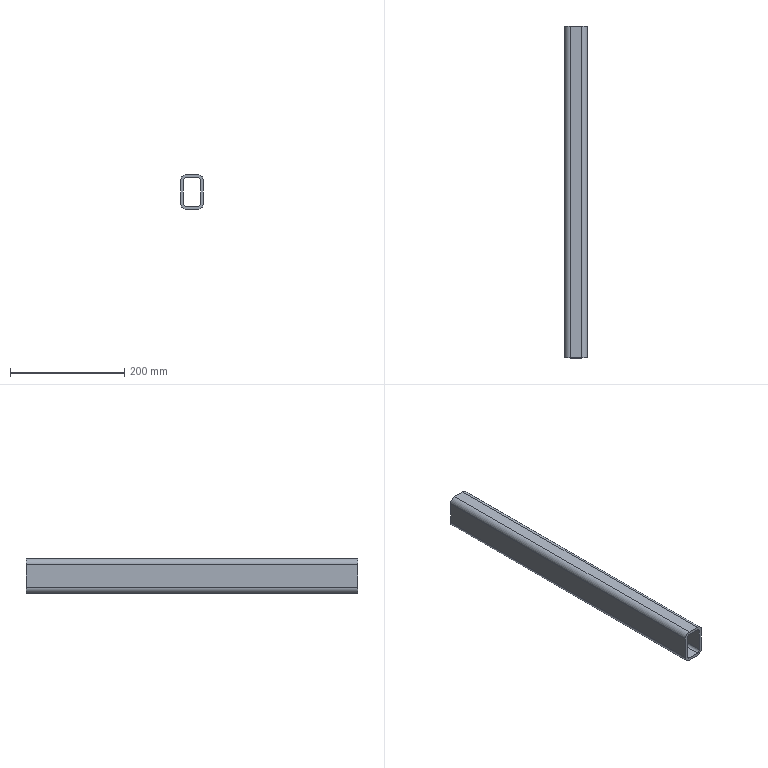Part | STEP file | HL4GD-1.30.109 base frame front crossmember--20251212 | 1 solid | 18 faces | box 40 x 580 x 60 mm | volume 484659 mm3 | plane 10 | cylinder 8 | commonest cylinder face diameters 10 x4 20 x4
STEP:
#1=CARTESIAN_POINT('',(0.,0.,0.));
#2=DIRECTION('',(0.,0.,1.));
#3=DIRECTION('',(1.,0.,0.));
#4=AXIS2_PLACEMENT_3D('',#1,#2,#3);
#5=CARTESIAN_POINT('',(2335.,1110.,410.));
#6=VERTEX_POINT('',#5);
#7=CARTESIAN_POINT('',(2330.,1110.,415.));
#8=VERTEX_POINT('',#7);
#9=CARTESIAN_POINT('',(2335.,1110.,415.));
#10=DIRECTION('',(0.,1.,0.));
#11=DIRECTION('',(-1.,0.,0.));
#12=AXIS2_PLACEMENT_3D('',#9,#10,#11);
#13=CIRCLE('',#12,5.);
#14=CARTESIAN_POINT('',(2335.,530.,415.));
#15=DIRECTION('',(0.,1.,0.));
#16=DIRECTION('',(-1.,0.,0.));
#17=AXIS2_PLACEMENT_3D('',#14,#15,#16);
#18=CYLINDRICAL_SURFACE('',#17,5.);
#19=CARTESIAN_POINT('',(0.,580.));
#20=DIRECTION('',(1.,0.));
#21=VECTOR('',#20,1.);
#22=LINE('',#19,#21);
#23=(GEOMETRIC_REPRESENTATION_CONTEXT(2)PARAMETRIC_REPRESENTATION_CONTEXT()REPRESENTATION_CONTEXT('',''));
#24=DEFINITIONAL_REPRESENTATION('',(#22),#23);
#25=PCURVE('',#18,#24);
#26=CARTESIAN_POINT('',(2148.93,1110.,281.07));
#27=DIRECTION('',(0.,1.,0.));
#28=DIRECTION('',(-1.,0.,0.));
#29=AXIS2_PLACEMENT_3D('',#26,#27,#28);
#30=PLANE('',#29);
#31=CARTESIAN_POINT('',(-186.07,133.93));
#32=DIRECTION('',(1.,0.));
#33=AXIS2_PLACEMENT_2D('',#31,#32);
#34=CIRCLE('',#33,5.);
#35=(GEOMETRIC_REPRESENTATION_CONTEXT(2)PARAMETRIC_REPRESENTATION_CONTEXT()REPRESENTATION_CONTEXT('',''));
#36=DEFINITIONAL_REPRESENTATION('',(#34),#35);
#37=PCURVE('',#30,#36);
#38=SURFACE_CURVE('',#13,(#25,#37),.PCURVE_S1.);
#39=EDGE_CURVE('',#6,#8,#38,.T.);
#40=ORIENTED_EDGE('',*,*,#39,.F.);
#41=CARTESIAN_POINT('',(2335.,530.,410.));
#42=VERTEX_POINT('',#41);
#43=CARTESIAN_POINT('',(2335.,530.,410.));
#44=DIRECTION('',(0.,1.,0.));
#45=VECTOR('',#44,1.);
#46=LINE('',#43,#45);
#47=CARTESIAN_POINT('',(4.712,0.));
#48=DIRECTION('',(0.,1.));
#49=VECTOR('',#48,1.);
#50=LINE('',#47,#49);
#51=(GEOMETRIC_REPRESENTATION_CONTEXT(2)PARAMETRIC_REPRESENTATION_CONTEXT()REPRESENTATION_CONTEXT('',''));
#52=DEFINITIONAL_REPRESENTATION('',(#50),#51);
#53=PCURVE('',#18,#52);
#54=CARTESIAN_POINT('',(2355.,530.,410.));
#55=DIRECTION('',(0.,0.,1.));
#56=DIRECTION('',(1.,0.,0.));
#57=AXIS2_PLACEMENT_3D('',#54,#55,#56);
#58=PLANE('',#57);
#59=CARTESIAN_POINT('',(-20.,0.));
#60=DIRECTION('',(0.,1.));
#61=VECTOR('',#60,1.);
#62=LINE('',#59,#61);
#63=(GEOMETRIC_REPRESENTATION_CONTEXT(2)PARAMETRIC_REPRESENTATION_CONTEXT()REPRESENTATION_CONTEXT('',''));
#64=DEFINITIONAL_REPRESENTATION('',(#62),#63);
#65=PCURVE('',#58,#64);
#66=SURFACE_CURVE('',#46,(#53,#65),.PCURVE_S1.);
#67=EDGE_CURVE('',#42,#6,#66,.T.);
#68=ORIENTED_EDGE('',*,*,#67,.F.);
#69=CARTESIAN_POINT('',(2330.,530.,415.));
#70=VERTEX_POINT('',#69);
#71=CARTESIAN_POINT('',(2335.,530.,415.));
#72=DIRECTION('',(0.,1.,0.));
#73=DIRECTION('',(-1.,0.,0.));
#74=AXIS2_PLACEMENT_3D('',#71,#72,#73);
#75=CIRCLE('',#74,5.);
#76=CARTESIAN_POINT('',(0.,0.));
#77=DIRECTION('',(1.,0.));
#78=VECTOR('',#77,1.);
#79=LINE('',#76,#78);
#80=(GEOMETRIC_REPRESENTATION_CONTEXT(2)PARAMETRIC_REPRESENTATION_CONTEXT()REPRESENTATION_CONTEXT('',''));
#81=DEFINITIONAL_REPRESENTATION('',(#79),#80);
#82=PCURVE('',#18,#81);
#83=CARTESIAN_POINT('',(2148.93,530.,281.07));
#84=DIRECTION('',(0.,1.,0.));
#85=DIRECTION('',(-1.,0.,0.));
#86=AXIS2_PLACEMENT_3D('',#83,#84,#85);
#87=PLANE('',#86);
#88=CARTESIAN_POINT('',(-186.07,133.93));
#89=DIRECTION('',(1.,0.));
#90=AXIS2_PLACEMENT_2D('',#88,#89);
#91=CIRCLE('',#90,5.);
#92=(GEOMETRIC_REPRESENTATION_CONTEXT(2)PARAMETRIC_REPRESENTATION_CONTEXT()REPRESENTATION_CONTEXT('',''));
#93=DEFINITIONAL_REPRESENTATION('',(#91),#92);
#94=PCURVE('',#87,#93);
#95=SURFACE_CURVE('',#75,(#82,#94),.PCURVE_S1.);
#96=EDGE_CURVE('',#42,#70,#95,.T.);
#97=ORIENTED_EDGE('',*,*,#96,.T.);
#98=CARTESIAN_POINT('',(2330.,530.,415.));
#99=DIRECTION('',(0.,1.,0.));
#100=VECTOR('',#99,1.);
#101=LINE('',#98,#100);
#102=CARTESIAN_POINT('',(6.283,0.));
#103=DIRECTION('',(0.,1.));
#104=VECTOR('',#103,1.);
#105=LINE('',#102,#104);
#106=(GEOMETRIC_REPRESENTATION_CONTEXT(2)PARAMETRIC_REPRESENTATION_CONTEXT()REPRESENTATION_CONTEXT('',''));
#107=DEFINITIONAL_REPRESENTATION('',(#105),#106);
#108=PCURVE('',#18,#107);
#109=CARTESIAN_POINT('',(2330.,530.,415.));
#110=DIRECTION('',(1.,0.,0.));
#111=DIRECTION('',(0.,0.,-1.));
#112=AXIS2_PLACEMENT_3D('',#109,#110,#111);
#113=PLANE('',#112);
#114=CARTESIAN_POINT('',(0.,0.));
#115=DIRECTION('',(0.,1.));
#116=VECTOR('',#115,1.);
#117=LINE('',#114,#116);
#118=(GEOMETRIC_REPRESENTATION_CONTEXT(2)PARAMETRIC_REPRESENTATION_CONTEXT()REPRESENTATION_CONTEXT('',''));
#119=DEFINITIONAL_REPRESENTATION('',(#117),#118);
#120=PCURVE('',#113,#119);
#121=SURFACE_CURVE('',#101,(#108,#120),.PCURVE_S1.);
#122=EDGE_CURVE('',#70,#8,#121,.T.);
#123=ORIENTED_EDGE('',*,*,#122,.T.);
#124=EDGE_LOOP('',(#40,#68,#97,#123));
#125=FACE_BOUND('',#124,.F.);
#126=ADVANCED_FACE('',(#125),#18,.F.);
#127=ORIENTED_EDGE('',*,*,#67,.F.);
#128=CARTESIAN_POINT('',(2355.,530.,410.));
#129=VERTEX_POINT('',#128);
#130=CARTESIAN_POINT('',(2355.,530.,410.));
#131=DIRECTION('',(1.,0.,0.));
#132=VECTOR('',#131,1.);
#133=LINE('',#130,#132);
#134=CARTESIAN_POINT('',(0.,0.));
#135=DIRECTION('',(1.,0.));
#136=VECTOR('',#135,1.);
#137=LINE('',#134,#136);
#138=(GEOMETRIC_REPRESENTATION_CONTEXT(2)PARAMETRIC_REPRESENTATION_CONTEXT()REPRESENTATION_CONTEXT('',''));
#139=DEFINITIONAL_REPRESENTATION('',(#137),#138);
#140=PCURVE('',#58,#139);
#141=CARTESIAN_POINT('',(-206.07,128.93));
#142=DIRECTION('',(-1.,0.));
#143=VECTOR('',#142,1.);
#144=LINE('',#141,#143);
#145=(GEOMETRIC_REPRESENTATION_CONTEXT(2)PARAMETRIC_REPRESENTATION_CONTEXT()REPRESENTATION_CONTEXT('',''));
#146=DEFINITIONAL_REPRESENTATION('',(#144),#145);
#147=PCURVE('',#87,#146);
#148=SURFACE_CURVE('',#133,(#140,#147),.PCURVE_S1.);
#149=EDGE_CURVE('',#42,#129,#148,.T.);
#150=ORIENTED_EDGE('',*,*,#149,.T.);
#151=CARTESIAN_POINT('',(2355.,1110.,410.));
#152=VERTEX_POINT('',#151);
#153=CARTESIAN_POINT('',(2355.,530.,410.));
#154=DIRECTION('',(0.,1.,0.));
#155=VECTOR('',#154,1.);
#156=LINE('',#153,#155);
#157=CARTESIAN_POINT('',(0.,0.));
#158=DIRECTION('',(0.,1.));
#159=VECTOR('',#158,1.);
#160=LINE('',#157,#159);
#161=(GEOMETRIC_REPRESENTATION_CONTEXT(2)PARAMETRIC_REPRESENTATION_CONTEXT()REPRESENTATION_CONTEXT('',''));
#162=DEFINITIONAL_REPRESENTATION('',(#160),#161);
#163=PCURVE('',#58,#162);
#164=CARTESIAN_POINT('',(2355.,530.,415.));
#165=DIRECTION('',(0.,1.,0.));
#166=DIRECTION('',(-1.,0.,0.));
#167=AXIS2_PLACEMENT_3D('',#164,#165,#166);
#168=CYLINDRICAL_SURFACE('',#167,5.);
#169=CARTESIAN_POINT('',(4.712,0.));
#170=DIRECTION('',(0.,1.));
#171=VECTOR('',#170,1.);
#172=LINE('',#169,#171);
#173=(GEOMETRIC_REPRESENTATION_CONTEXT(2)PARAMETRIC_REPRESENTATION_CONTEXT()REPRESENTATION_CONTEXT('',''));
#174=DEFINITIONAL_REPRESENTATION('',(#172),#173);
#175=PCURVE('',#168,#174);
#176=SURFACE_CURVE('',#156,(#163,#175),.PCURVE_S1.);
#177=EDGE_CURVE('',#129,#152,#176,.T.);
#178=ORIENTED_EDGE('',*,*,#177,.T.);
#179=CARTESIAN_POINT('',(2148.93,1110.,410.));
#180=DIRECTION('',(1.,0.,0.));
#181=VECTOR('',#180,1.);
#182=LINE('',#179,#181);
#183=CARTESIAN_POINT('',(-206.07,580.));
#184=DIRECTION('',(1.,0.));
#185=VECTOR('',#184,1.);
#186=LINE('',#183,#185);
#187=(GEOMETRIC_REPRESENTATION_CONTEXT(2)PARAMETRIC_REPRESENTATION_CONTEXT()REPRESENTATION_CONTEXT('',''));
#188=DEFINITIONAL_REPRESENTATION('',(#186),#187);
#189=PCURVE('',#58,#188);
#190=CARTESIAN_POINT('',(0.,128.93));
#191=DIRECTION('',(-1.,0.));
#192=VECTOR('',#191,1.);
#193=LINE('',#190,#192);
#194=(GEOMETRIC_REPRESENTATION_CONTEXT(2)PARAMETRIC_REPRESENTATION_CONTEXT()REPRESENTATION_CONTEXT('',''));
#195=DEFINITIONAL_REPRESENTATION('',(#193),#194);
#196=PCURVE('',#30,#195);
#197=SURFACE_CURVE('',#182,(#189,#196),.PCURVE_S1.);
#198=EDGE_CURVE('',#6,#152,#197,.T.);
#199=ORIENTED_EDGE('',*,*,#198,.F.);
#200=EDGE_LOOP('',(#127,#150,#178,#199));
#201=FACE_BOUND('',#200,.T.);
#202=ADVANCED_FACE('',(#201),#58,.T.);
#203=CARTESIAN_POINT('',(2360.,1110.,415.));
#204=VERTEX_POINT('',#203);
#205=CARTESIAN_POINT('',(2355.,1110.,415.));
#206=DIRECTION('',(0.,-1.,0.));
#207=DIRECTION('',(-1.,0.,0.));
#208=AXIS2_PLACEMENT_3D('',#205,#206,#207);
#209=CIRCLE('',#208,5.);
#210=CARTESIAN_POINT('',(6.283,580.));
#211=DIRECTION('',(-1.,0.));
#212=VECTOR('',#211,1.);
#213=LINE('',#210,#212);
#214=(GEOMETRIC_REPRESENTATION_CONTEXT(2)PARAMETRIC_REPRESENTATION_CONTEXT()REPRESENTATION_CONTEXT('',''));
#215=DEFINITIONAL_REPRESENTATION('',(#213),#214);
#216=PCURVE('',#168,#215);
#217=CARTESIAN_POINT('',(-201.07,133.93));
#218=CARTESIAN_POINT('',(-201.07,125.27));
#219=CARTESIAN_POINT('',(-208.57,129.6));
#220=CARTESIAN_POINT('',(-216.07,133.93));
#221=CARTESIAN_POINT('',(-208.57,138.261));
#222=CARTESIAN_POINT('',(-201.07,142.591));
#223=CARTESIAN_POINT('',(-201.07,133.93));
#224=(BOUNDED_CURVE()B_SPLINE_CURVE(2,(#217,#218,#219,#220,#221,#222,#223),.UNSPECIFIED.,.T.,.F.)B_SPLINE_CURVE_WITH_KNOTS((1,2,2,2,2,1),(-2.094,0.,2.094,4.189,6.283,8.378),.UNSPECIFIED.)CURVE()GEOMETRIC_REPRESENTATION_ITEM()RATIONAL_B_SPLINE_CURVE((1.,0.5,1.,0.5,1.,0.5,1.))REPRESENTATION_ITEM(''));
#225=(GEOMETRIC_REPRESENTATION_CONTEXT(2)PARAMETRIC_REPRESENTATION_CONTEXT()REPRESENTATION_CONTEXT('',''));
#226=DEFINITIONAL_REPRESENTATION('',(#224),#225);
#227=PCURVE('',#30,#226);
#228=SURFACE_CURVE('',#209,(#216,#227),.PCURVE_S1.);
#229=EDGE_CURVE('',#152,#204,#228,.T.);
#230=ORIENTED_EDGE('',*,*,#229,.T.);
#231=CARTESIAN_POINT('',(2360.,530.,415.));
#232=VERTEX_POINT('',#231);
#233=CARTESIAN_POINT('',(2360.,530.,415.));
#234=DIRECTION('',(0.,1.,0.));
#235=VECTOR('',#234,1.);
#236=LINE('',#233,#235);
#237=CARTESIAN_POINT('',(3.142,0.));
#238=DIRECTION('',(0.,1.));
#239=VECTOR('',#238,1.);
#240=LINE('',#237,#239);
#241=(GEOMETRIC_REPRESENTATION_CONTEXT(2)PARAMETRIC_REPRESENTATION_CONTEXT()REPRESENTATION_CONTEXT('',''));
#242=DEFINITIONAL_REPRESENTATION('',(#240),#241);
#243=PCURVE('',#168,#242);
#244=CARTESIAN_POINT('',(2360.,530.,455.));
#245=DIRECTION('',(-1.,0.,0.));
#246=DIRECTION('',(0.,0.,1.));
#247=AXIS2_PLACEMENT_3D('',#244,#245,#246);
#248=PLANE('',#247);
#249=CARTESIAN_POINT('',(-40.,0.));
#250=DIRECTION('',(0.,1.));
#251=VECTOR('',#250,1.);
#252=LINE('',#249,#251);
#253=(GEOMETRIC_REPRESENTATION_CONTEXT(2)PARAMETRIC_REPRESENTATION_CONTEXT()REPRESENTATION_CONTEXT('',''));
#254=DEFINITIONAL_REPRESENTATION('',(#252),#253);
#255=PCURVE('',#248,#254);
#256=SURFACE_CURVE('',#236,(#243,#255),.PCURVE_S1.);
#257=EDGE_CURVE('',#232,#204,#256,.T.);
#258=ORIENTED_EDGE('',*,*,#257,.F.);
#259=CARTESIAN_POINT('',(2355.,530.,415.));
#260=DIRECTION('',(0.,-1.,0.));
#261=DIRECTION('',(-1.,0.,0.));
#262=AXIS2_PLACEMENT_3D('',#259,#260,#261);
#263=CIRCLE('',#262,5.);
#264=CARTESIAN_POINT('',(6.283,0.));
#265=DIRECTION('',(-1.,0.));
#266=VECTOR('',#265,1.);
#267=LINE('',#264,#266);
#268=(GEOMETRIC_REPRESENTATION_CONTEXT(2)PARAMETRIC_REPRESENTATION_CONTEXT()REPRESENTATION_CONTEXT('',''));
#269=DEFINITIONAL_REPRESENTATION('',(#267),#268);
#270=PCURVE('',#168,#269);
#271=CARTESIAN_POINT('',(-201.07,133.93));
#272=CARTESIAN_POINT('',(-201.07,125.27));
#273=CARTESIAN_POINT('',(-208.57,129.6));
#274=CARTESIAN_POINT('',(-216.07,133.93));
#275=CARTESIAN_POINT('',(-208.57,138.261));
#276=CARTESIAN_POINT('',(-201.07,142.591));
#277=CARTESIAN_POINT('',(-201.07,133.93));
#278=(BOUNDED_CURVE()B_SPLINE_CURVE(2,(#271,#272,#273,#274,#275,#276,#277),.UNSPECIFIED.,.T.,.F.)B_SPLINE_CURVE_WITH_KNOTS((1,2,2,2,2,1),(-2.094,0.,2.094,4.189,6.283,8.378),.UNSPECIFIED.)CURVE()GEOMETRIC_REPRESENTATION_ITEM()RATIONAL_B_SPLINE_CURVE((1.,0.5,1.,0.5,1.,0.5,1.))REPRESENTATION_ITEM(''));
#279=(GEOMETRIC_REPRESENTATION_CONTEXT(2)PARAMETRIC_REPRESENTATION_CONTEXT()REPRESENTATION_CONTEXT('',''));
#280=DEFINITIONAL_REPRESENTATION('',(#278),#279);
#281=PCURVE('',#87,#280);
#282=SURFACE_CURVE('',#263,(#270,#281),.PCURVE_S1.);
#283=EDGE_CURVE('',#129,#232,#282,.T.);
#284=ORIENTED_EDGE('',*,*,#283,.F.);
#285=ORIENTED_EDGE('',*,*,#177,.T.);
#286=EDGE_LOOP('',(#230,#258,#284,#285));
#287=FACE_BOUND('',#286,.F.);
#288=ADVANCED_FACE('',(#287),#168,.F.);
#289=ORIENTED_EDGE('',*,*,#257,.F.);
#290=CARTESIAN_POINT('',(2360.,530.,455.));
#291=VERTEX_POINT('',#290);
#292=CARTESIAN_POINT('',(2360.,530.,455.));
#293=DIRECTION('',(0.,0.,-1.));
#294=VECTOR('',#293,1.);
#295=LINE('',#292,#294);
#296=CARTESIAN_POINT('',(0.,0.));
#297=DIRECTION('',(-1.,0.));
#298=VECTOR('',#297,1.);
#299=LINE('',#296,#298);
#300=(GEOMETRIC_REPRESENTATION_CONTEXT(2)PARAMETRIC_REPRESENTATION_CONTEXT()REPRESENTATION_CONTEXT('',''));
#301=DEFINITIONAL_REPRESENTATION('',(#299),#300);
#302=PCURVE('',#248,#301);
#303=CARTESIAN_POINT('',(-211.07,173.93));
#304=DIRECTION('',(0.,-1.));
#305=VECTOR('',#304,1.);
#306=LINE('',#303,#305);
#307=(GEOMETRIC_REPRESENTATION_CONTEXT(2)PARAMETRIC_REPRESENTATION_CONTEXT()REPRESENTATION_CONTEXT('',''));
#308=DEFINITIONAL_REPRESENTATION('',(#306),#307);
#309=PCURVE('',#87,#308);
#310=SURFACE_CURVE('',#295,(#302,#309),.PCURVE_S1.);
#311=EDGE_CURVE('',#291,#232,#310,.T.);
#312=ORIENTED_EDGE('',*,*,#311,.F.);
#313=CARTESIAN_POINT('',(2360.,1110.,455.));
#314=VERTEX_POINT('',#313);
#315=CARTESIAN_POINT('',(2360.,530.,455.));
#316=DIRECTION('',(0.,1.,0.));
#317=VECTOR('',#316,1.);
#318=LINE('',#315,#317);
#319=CARTESIAN_POINT('',(0.,0.));
#320=DIRECTION('',(0.,1.));
#321=VECTOR('',#320,1.);
#322=LINE('',#319,#321);
#323=(GEOMETRIC_REPRESENTATION_CONTEXT(2)PARAMETRIC_REPRESENTATION_CONTEXT()REPRESENTATION_CONTEXT('',''));
#324=DEFINITIONAL_REPRESENTATION('',(#322),#323);
#325=PCURVE('',#248,#324);
#326=CARTESIAN_POINT('',(2355.,530.,455.));
#327=DIRECTION('',(0.,1.,0.));
#328=DIRECTION('',(-1.,0.,0.));
#329=AXIS2_PLACEMENT_3D('',#326,#327,#328);
#330=CYLINDRICAL_SURFACE('',#329,5.);
#331=CARTESIAN_POINT('',(3.142,0.));
#332=DIRECTION('',(0.,1.));
#333=VECTOR('',#332,1.);
#334=LINE('',#331,#333);
#335=(GEOMETRIC_REPRESENTATION_CONTEXT(2)PARAMETRIC_REPRESENTATION_CONTEXT()REPRESENTATION_CONTEXT('',''));
#336=DEFINITIONAL_REPRESENTATION('',(#334),#335);
#337=PCURVE('',#330,#336);
#338=SURFACE_CURVE('',#318,(#325,#337),.PCURVE_S1.);
#339=EDGE_CURVE('',#291,#314,#338,.T.);
#340=ORIENTED_EDGE('',*,*,#339,.T.);
#341=CARTESIAN_POINT('',(2360.,1110.,281.07));
#342=DIRECTION('',(0.,0.,-1.));
#343=VECTOR('',#342,1.);
#344=LINE('',#341,#343);
#345=CARTESIAN_POINT('',(-173.93,580.));
#346=DIRECTION('',(-1.,0.));
#347=VECTOR('',#346,1.);
#348=LINE('',#345,#347);
#349=(GEOMETRIC_REPRESENTATION_CONTEXT(2)PARAMETRIC_REPRESENTATION_CONTEXT()REPRESENTATION_CONTEXT('',''));
#350=DEFINITIONAL_REPRESENTATION('',(#348),#349);
#351=PCURVE('',#248,#350);
#352=CARTESIAN_POINT('',(-211.07,0.));
#353=DIRECTION('',(0.,-1.));
#354=VECTOR('',#353,1.);
#355=LINE('',#352,#354);
#356=(GEOMETRIC_REPRESENTATION_CONTEXT(2)PARAMETRIC_REPRESENTATION_CONTEXT()REPRESENTATION_CONTEXT('',''));
#357=DEFINITIONAL_REPRESENTATION('',(#355),#356);
#358=PCURVE('',#30,#357);
#359=SURFACE_CURVE('',#344,(#351,#358),.PCURVE_S1.);
#360=EDGE_CURVE('',#314,#204,#359,.T.);
#361=ORIENTED_EDGE('',*,*,#360,.T.);
#362=EDGE_LOOP('',(#289,#312,#340,#361));
#363=FACE_BOUND('',#362,.T.);
#364=ADVANCED_FACE('',(#363),#248,.T.);
#365=CARTESIAN_POINT('',(2355.,1110.,460.));
#366=VERTEX_POINT('',#365);
#367=CARTESIAN_POINT('',(2355.,1110.,455.));
#368=DIRECTION('',(0.,1.,0.));
#369=DIRECTION('',(-1.,0.,0.));
#370=AXIS2_PLACEMENT_3D('',#367,#368,#369);
#371=CIRCLE('',#370,5.);
#372=CARTESIAN_POINT('',(0.,580.));
#373=DIRECTION('',(1.,0.));
#374=VECTOR('',#373,1.);
#375=LINE('',#372,#374);
#376=(GEOMETRIC_REPRESENTATION_CONTEXT(2)PARAMETRIC_REPRESENTATION_CONTEXT()REPRESENTATION_CONTEXT('',''));
#377=DEFINITIONAL_REPRESENTATION('',(#375),#376);
#378=PCURVE('',#330,#377);
#379=CARTESIAN_POINT('',(-206.07,173.93));
#380=DIRECTION('',(1.,0.));
#381=AXIS2_PLACEMENT_2D('',#379,#380);
#382=CIRCLE('',#381,5.);
#383=(GEOMETRIC_REPRESENTATION_CONTEXT(2)PARAMETRIC_REPRESENTATION_CONTEXT()REPRESENTATION_CONTEXT('',''));
#384=DEFINITIONAL_REPRESENTATION('',(#382),#383);
#385=PCURVE('',#30,#384);
#386=SURFACE_CURVE('',#371,(#378,#385),.PCURVE_S1.);
#387=EDGE_CURVE('',#366,#314,#386,.T.);
#388=ORIENTED_EDGE('',*,*,#387,.F.);
#389=CARTESIAN_POINT('',(2355.,530.,460.));
#390=VERTEX_POINT('',#389);
#391=CARTESIAN_POINT('',(2355.,530.,460.));
#392=DIRECTION('',(0.,1.,0.));
#393=VECTOR('',#392,1.);
#394=LINE('',#391,#393);
#395=CARTESIAN_POINT('',(1.571,0.));
#396=DIRECTION('',(0.,1.));
#397=VECTOR('',#396,1.);
#398=LINE('',#395,#397);
#399=(GEOMETRIC_REPRESENTATION_CONTEXT(2)PARAMETRIC_REPRESENTATION_CONTEXT()REPRESENTATION_CONTEXT('',''));
#400=DEFINITIONAL_REPRESENTATION('',(#398),#399);
#401=PCURVE('',#330,#400);
#402=CARTESIAN_POINT('',(2335.,530.,460.));
#403=DIRECTION('',(0.,0.,-1.));
#404=DIRECTION('',(-1.,0.,0.));
#405=AXIS2_PLACEMENT_3D('',#402,#403,#404);
#406=PLANE('',#405);
#407=CARTESIAN_POINT('',(-20.,0.));
#408=DIRECTION('',(0.,1.));
#409=VECTOR('',#408,1.);
#410=LINE('',#407,#409);
#411=(GEOMETRIC_REPRESENTATION_CONTEXT(2)PARAMETRIC_REPRESENTATION_CONTEXT()REPRESENTATION_CONTEXT('',''));
#412=DEFINITIONAL_REPRESENTATION('',(#410),#411);
#413=PCURVE('',#406,#412);
#414=SURFACE_CURVE('',#394,(#401,#413),.PCURVE_S1.);
#415=EDGE_CURVE('',#390,#366,#414,.T.);
#416=ORIENTED_EDGE('',*,*,#415,.F.);
#417=CARTESIAN_POINT('',(2355.,530.,455.));
#418=DIRECTION('',(0.,1.,0.));
#419=DIRECTION('',(-1.,0.,0.));
#420=AXIS2_PLACEMENT_3D('',#417,#418,#419);
#421=CIRCLE('',#420,5.);
#422=CARTESIAN_POINT('',(0.,0.));
#423=DIRECTION('',(1.,0.));
#424=VECTOR('',#423,1.);
#425=LINE('',#422,#424);
#426=(GEOMETRIC_REPRESENTATION_CONTEXT(2)PARAMETRIC_REPRESENTATION_CONTEXT()REPRESENTATION_CONTEXT('',''));
#427=DEFINITIONAL_REPRESENTATION('',(#425),#426);
#428=PCURVE('',#330,#427);
#429=CARTESIAN_POINT('',(-206.07,173.93));
#430=DIRECTION('',(1.,0.));
#431=AXIS2_PLACEMENT_2D('',#429,#430);
#432=CIRCLE('',#431,5.);
#433=(GEOMETRIC_REPRESENTATION_CONTEXT(2)PARAMETRIC_REPRESENTATION_CONTEXT()REPRESENTATION_CONTEXT('',''));
#434=DEFINITIONAL_REPRESENTATION('',(#432),#433);
#435=PCURVE('',#87,#434);
#436=SURFACE_CURVE('',#421,(#428,#435),.PCURVE_S1.);
#437=EDGE_CURVE('',#390,#291,#436,.T.);
#438=ORIENTED_EDGE('',*,*,#437,.T.);
#439=ORIENTED_EDGE('',*,*,#339,.T.);
#440=EDGE_LOOP('',(#388,#416,#438,#439));
#441=FACE_BOUND('',#440,.F.);
#442=ADVANCED_FACE('',(#441),#330,.F.);
#443=ORIENTED_EDGE('',*,*,#415,.F.);
#444=CARTESIAN_POINT('',(2335.,530.,460.));
#445=VERTEX_POINT('',#444);
#446=CARTESIAN_POINT('',(2335.,530.,460.));
#447=DIRECTION('',(1.,0.,0.));
#448=VECTOR('',#447,1.);
#449=LINE('',#446,#448);
#450=CARTESIAN_POINT('',(0.,0.));
#451=DIRECTION('',(-1.,0.));
#452=VECTOR('',#451,1.);
#453=LINE('',#450,#452);
#454=(GEOMETRIC_REPRESENTATION_CONTEXT(2)PARAMETRIC_REPRESENTATION_CONTEXT()REPRESENTATION_CONTEXT('',''));
#455=DEFINITIONAL_REPRESENTATION('',(#453),#454);
#456=PCURVE('',#406,#455);
#457=CARTESIAN_POINT('',(-186.07,178.93));
#458=DIRECTION('',(-1.,0.));
#459=VECTOR('',#458,1.);
#460=LINE('',#457,#459);
#461=(GEOMETRIC_REPRESENTATION_CONTEXT(2)PARAMETRIC_REPRESENTATION_CONTEXT()REPRESENTATION_CONTEXT('',''));
#462=DEFINITIONAL_REPRESENTATION('',(#460),#461);
#463=PCURVE('',#87,#462);
#464=SURFACE_CURVE('',#449,(#456,#463),.PCURVE_S1.);
#465=EDGE_CURVE('',#445,#390,#464,.T.);
#466=ORIENTED_EDGE('',*,*,#465,.F.);
#467=CARTESIAN_POINT('',(2335.,1110.,460.));
#468=VERTEX_POINT('',#467);
#469=CARTESIAN_POINT('',(2335.,530.,460.));
#470=DIRECTION('',(0.,1.,0.));
#471=VECTOR('',#470,1.);
#472=LINE('',#469,#471);
#473=CARTESIAN_POINT('',(0.,0.));
#474=DIRECTION('',(0.,1.));
#475=VECTOR('',#474,1.);
#476=LINE('',#473,#475);
#477=(GEOMETRIC_REPRESENTATION_CONTEXT(2)PARAMETRIC_REPRESENTATION_CONTEXT()REPRESENTATION_CONTEXT('',''));
#478=DEFINITIONAL_REPRESENTATION('',(#476),#477);
#479=PCURVE('',#406,#478);
#480=CARTESIAN_POINT('',(2335.,530.,455.));
#481=DIRECTION('',(0.,1.,0.));
#482=DIRECTION('',(-1.,0.,0.));
#483=AXIS2_PLACEMENT_3D('',#480,#481,#482);
#484=CYLINDRICAL_SURFACE('',#483,5.);
#485=CARTESIAN_POINT('',(1.571,0.));
#486=DIRECTION('',(0.,1.));
#487=VECTOR('',#486,1.);
#488=LINE('',#485,#487);
#489=(GEOMETRIC_REPRESENTATION_CONTEXT(2)PARAMETRIC_REPRESENTATION_CONTEXT()REPRESENTATION_CONTEXT('',''));
#490=DEFINITIONAL_REPRESENTATION('',(#488),#489);
#491=PCURVE('',#484,#490);
#492=SURFACE_CURVE('',#472,(#479,#491),.PCURVE_S1.);
#493=EDGE_CURVE('',#445,#468,#492,.T.);
#494=ORIENTED_EDGE('',*,*,#493,.T.);
#495=CARTESIAN_POINT('',(2148.93,1110.,460.));
#496=DIRECTION('',(1.,0.,0.));
#497=VECTOR('',#496,1.);
#498=LINE('',#495,#497);
#499=CARTESIAN_POINT('',(186.07,580.));
#500=DIRECTION('',(-1.,0.));
#501=VECTOR('',#500,1.);
#502=LINE('',#499,#501);
#503=(GEOMETRIC_REPRESENTATION_CONTEXT(2)PARAMETRIC_REPRESENTATION_CONTEXT()REPRESENTATION_CONTEXT('',''));
#504=DEFINITIONAL_REPRESENTATION('',(#502),#503);
#505=PCURVE('',#406,#504);
#506=CARTESIAN_POINT('',(0.,178.93));
#507=DIRECTION('',(-1.,0.));
#508=VECTOR('',#507,1.);
#509=LINE('',#506,#508);
#510=(GEOMETRIC_REPRESENTATION_CONTEXT(2)PARAMETRIC_REPRESENTATION_CONTEXT()REPRESENTATION_CONTEXT('',''));
#511=DEFINITIONAL_REPRESENTATION('',(#509),#510);
#512=PCURVE('',#30,#511);
#513=SURFACE_CURVE('',#498,(#505,#512),.PCURVE_S1.);
#514=EDGE_CURVE('',#468,#366,#513,.T.);
#515=ORIENTED_EDGE('',*,*,#514,.T.);
#516=EDGE_LOOP('',(#443,#466,#494,#515));
#517=FACE_BOUND('',#516,.T.);
#518=ADVANCED_FACE('',(#517),#406,.T.);
#519=CARTESIAN_POINT('',(2330.,1110.,455.));
#520=VERTEX_POINT('',#519);
#521=CARTESIAN_POINT('',(2335.,1110.,455.));
#522=DIRECTION('',(0.,-1.,0.));
#523=DIRECTION('',(-1.,0.,0.));
#524=AXIS2_PLACEMENT_3D('',#521,#522,#523);
#525=CIRCLE('',#524,5.);
#526=CARTESIAN_POINT('',(6.283,580.));
#527=DIRECTION('',(-1.,0.));
#528=VECTOR('',#527,1.);
#529=LINE('',#526,#528);
#530=(GEOMETRIC_REPRESENTATION_CONTEXT(2)PARAMETRIC_REPRESENTATION_CONTEXT()REPRESENTATION_CONTEXT('',''));
#531=DEFINITIONAL_REPRESENTATION('',(#529),#530);
#532=PCURVE('',#484,#531);
#533=CARTESIAN_POINT('',(-181.07,173.93));
#534=CARTESIAN_POINT('',(-181.07,165.27));
#535=CARTESIAN_POINT('',(-188.57,169.6));
#536=CARTESIAN_POINT('',(-196.07,173.93));
#537=CARTESIAN_POINT('',(-188.57,178.261));
#538=CARTESIAN_POINT('',(-181.07,182.591));
#539=CARTESIAN_POINT('',(-181.07,173.93));
#540=(BOUNDED_CURVE()B_SPLINE_CURVE(2,(#533,#534,#535,#536,#537,#538,#539),.UNSPECIFIED.,.T.,.F.)B_SPLINE_CURVE_WITH_KNOTS((1,2,2,2,2,1),(-2.094,0.,2.094,4.189,6.283,8.378),.UNSPECIFIED.)CURVE()GEOMETRIC_REPRESENTATION_ITEM()RATIONAL_B_SPLINE_CURVE((1.,0.5,1.,0.5,1.,0.5,1.))REPRESENTATION_ITEM(''));
#541=(GEOMETRIC_REPRESENTATION_CONTEXT(2)PARAMETRIC_REPRESENTATION_CONTEXT()REPRESENTATION_CONTEXT('',''));
#542=DEFINITIONAL_REPRESENTATION('',(#540),#541);
#543=PCURVE('',#30,#542);
#544=SURFACE_CURVE('',#525,(#532,#543),.PCURVE_S1.);
#545=EDGE_CURVE('',#468,#520,#544,.T.);
#546=ORIENTED_EDGE('',*,*,#545,.T.);
#547=CARTESIAN_POINT('',(2330.,530.,455.));
#548=VERTEX_POINT('',#547);
#549=CARTESIAN_POINT('',(2330.,530.,455.));
#550=DIRECTION('',(0.,1.,0.));
#551=VECTOR('',#550,1.);
#552=LINE('',#549,#551);
#553=CARTESIAN_POINT('',(0.,0.));
#554=DIRECTION('',(0.,1.));
#555=VECTOR('',#554,1.);
#556=LINE('',#553,#555);
#557=(GEOMETRIC_REPRESENTATION_CONTEXT(2)PARAMETRIC_REPRESENTATION_CONTEXT()REPRESENTATION_CONTEXT('',''));
#558=DEFINITIONAL_REPRESENTATION('',(#556),#557);
#559=PCURVE('',#484,#558);
#560=CARTESIAN_POINT('',(-40.,0.));
#561=DIRECTION('',(0.,1.));
#562=VECTOR('',#561,1.);
#563=LINE('',#560,#562);
#564=(GEOMETRIC_REPRESENTATION_CONTEXT(2)PARAMETRIC_REPRESENTATION_CONTEXT()REPRESENTATION_CONTEXT('',''));
#565=DEFINITIONAL_REPRESENTATION('',(#563),#564);
#566=PCURVE('',#113,#565);
#567=SURFACE_CURVE('',#552,(#559,#566),.PCURVE_S1.);
#568=EDGE_CURVE('',#548,#520,#567,.T.);
#569=ORIENTED_EDGE('',*,*,#568,.F.);
#570=CARTESIAN_POINT('',(2335.,530.,455.));
#571=DIRECTION('',(0.,-1.,0.));
#572=DIRECTION('',(-1.,0.,0.));
#573=AXIS2_PLACEMENT_3D('',#570,#571,#572);
#574=CIRCLE('',#573,5.);
#575=CARTESIAN_POINT('',(6.283,0.));
#576=DIRECTION('',(-1.,0.));
#577=VECTOR('',#576,1.);
#578=LINE('',#575,#577);
#579=(GEOMETRIC_REPRESENTATION_CONTEXT(2)PARAMETRIC_REPRESENTATION_CONTEXT()REPRESENTATION_CONTEXT('',''));
#580=DEFINITIONAL_REPRESENTATION('',(#578),#579);
#581=PCURVE('',#484,#580);
#582=CARTESIAN_POINT('',(-181.07,173.93));
#583=CARTESIAN_POINT('',(-181.07,165.27));
#584=CARTESIAN_POINT('',(-188.57,169.6));
#585=CARTESIAN_POINT('',(-196.07,173.93));
#586=CARTESIAN_POINT('',(-188.57,178.261));
#587=CARTESIAN_POINT('',(-181.07,182.591));
#588=CARTESIAN_POINT('',(-181.07,173.93));
#589=(BOUNDED_CURVE()B_SPLINE_CURVE(2,(#582,#583,#584,#585,#586,#587,#588),.UNSPECIFIED.,.T.,.F.)B_SPLINE_CURVE_WITH_KNOTS((1,2,2,2,2,1),(-2.094,0.,2.094,4.189,6.283,8.378),.UNSPECIFIED.)CURVE()GEOMETRIC_REPRESENTATION_ITEM()RATIONAL_B_SPLINE_CURVE((1.,0.5,1.,0.5,1.,0.5,1.))REPRESENTATION_ITEM(''));
#590=(GEOMETRIC_REPRESENTATION_CONTEXT(2)PARAMETRIC_REPRESENTATION_CONTEXT()REPRESENTATION_CONTEXT('',''));
#591=DEFINITIONAL_REPRESENTATION('',(#589),#590);
#592=PCURVE('',#87,#591);
#593=SURFACE_CURVE('',#574,(#581,#592),.PCURVE_S1.);
#594=EDGE_CURVE('',#445,#548,#593,.T.);
#595=ORIENTED_EDGE('',*,*,#594,.F.);
#596=ORIENTED_EDGE('',*,*,#493,.T.);
#597=EDGE_LOOP('',(#546,#569,#595,#596));
#598=FACE_BOUND('',#597,.F.);
#599=ADVANCED_FACE('',(#598),#484,.F.);
#600=CARTESIAN_POINT('',(2365.,530.,455.));
#601=VERTEX_POINT('',#600);
#602=CARTESIAN_POINT('',(2365.,1110.,455.));
#603=VERTEX_POINT('',#602);
#604=CARTESIAN_POINT('',(2365.,530.,455.));
#605=DIRECTION('',(0.,1.,0.));
#606=VECTOR('',#605,1.);
#607=LINE('',#604,#606);
#608=CARTESIAN_POINT('',(2365.,530.,455.));
#609=DIRECTION('',(-1.,0.,0.));
#610=DIRECTION('',(0.,0.,1.));
#611=AXIS2_PLACEMENT_3D('',#608,#609,#610);
#612=PLANE('',#611);
#613=CARTESIAN_POINT('',(0.,0.));
#614=DIRECTION('',(0.,1.));
#615=VECTOR('',#614,1.);
#616=LINE('',#613,#615);
#617=(GEOMETRIC_REPRESENTATION_CONTEXT(2)PARAMETRIC_REPRESENTATION_CONTEXT()REPRESENTATION_CONTEXT('',''));
#618=DEFINITIONAL_REPRESENTATION('',(#616),#617);
#619=PCURVE('',#612,#618);
#620=CARTESIAN_POINT('',(2355.,530.,455.));
#621=DIRECTION('',(0.,1.,0.));
#622=DIRECTION('',(-1.,0.,0.));
#623=AXIS2_PLACEMENT_3D('',#620,#621,#622);
#624=CYLINDRICAL_SURFACE('',#623,10.);
#625=CARTESIAN_POINT('',(3.142,0.));
#626=DIRECTION('',(0.,1.));
#627=VECTOR('',#626,1.);
#628=LINE('',#625,#627);
#629=(GEOMETRIC_REPRESENTATION_CONTEXT(2)PARAMETRIC_REPRESENTATION_CONTEXT()REPRESENTATION_CONTEXT('',''));
#630=DEFINITIONAL_REPRESENTATION('',(#628),#629);
#631=PCURVE('',#624,#630);
#632=SURFACE_CURVE('',#607,(#619,#631),.PCURVE_S1.);
#633=EDGE_CURVE('',#601,#603,#632,.T.);
#634=ORIENTED_EDGE('',*,*,#633,.F.);
#635=CARTESIAN_POINT('',(2365.,530.,415.));
#636=VERTEX_POINT('',#635);
#637=CARTESIAN_POINT('',(2365.,530.,455.));
#638=DIRECTION('',(0.,0.,1.));
#639=VECTOR('',#638,1.);
#640=LINE('',#637,#639);
#641=CARTESIAN_POINT('',(0.,0.));
#642=DIRECTION('',(1.,0.));
#643=VECTOR('',#642,1.);
#644=LINE('',#641,#643);
#645=(GEOMETRIC_REPRESENTATION_CONTEXT(2)PARAMETRIC_REPRESENTATION_CONTEXT()REPRESENTATION_CONTEXT('',''));
#646=DEFINITIONAL_REPRESENTATION('',(#644),#645);
#647=PCURVE('',#612,#646);
#648=CARTESIAN_POINT('',(-216.07,173.93));
#649=DIRECTION('',(0.,1.));
#650=VECTOR('',#649,1.);
#651=LINE('',#648,#650);
#652=(GEOMETRIC_REPRESENTATION_CONTEXT(2)PARAMETRIC_REPRESENTATION_CONTEXT()REPRESENTATION_CONTEXT('',''));
#653=DEFINITIONAL_REPRESENTATION('',(#651),#652);
#654=PCURVE('',#87,#653);
#655=SURFACE_CURVE('',#640,(#647,#654),.PCURVE_S1.);
#656=EDGE_CURVE('',#636,#601,#655,.T.);
#657=ORIENTED_EDGE('',*,*,#656,.F.);
#658=CARTESIAN_POINT('',(2365.,1110.,415.));
#659=VERTEX_POINT('',#658);
#660=CARTESIAN_POINT('',(2365.,530.,415.));
#661=DIRECTION('',(0.,1.,0.));
#662=VECTOR('',#661,1.);
#663=LINE('',#660,#662);
#664=CARTESIAN_POINT('',(-40.,0.));
#665=DIRECTION('',(0.,1.));
#666=VECTOR('',#665,1.);
#667=LINE('',#664,#666);
#668=(GEOMETRIC_REPRESENTATION_CONTEXT(2)PARAMETRIC_REPRESENTATION_CONTEXT()REPRESENTATION_CONTEXT('',''));
#669=DEFINITIONAL_REPRESENTATION('',(#667),#668);
#670=PCURVE('',#612,#669);
#671=CARTESIAN_POINT('',(2355.,530.,415.));
#672=DIRECTION('',(0.,1.,0.));
#673=DIRECTION('',(-1.,0.,0.));
#674=AXIS2_PLACEMENT_3D('',#671,#672,#673);
#675=CYLINDRICAL_SURFACE('',#674,10.);
#676=CARTESIAN_POINT('',(3.142,0.));
#677=DIRECTION('',(0.,1.));
#678=VECTOR('',#677,1.);
#679=LINE('',#676,#678);
#680=(GEOMETRIC_REPRESENTATION_CONTEXT(2)PARAMETRIC_REPRESENTATION_CONTEXT()REPRESENTATION_CONTEXT('',''));
#681=DEFINITIONAL_REPRESENTATION('',(#679),#680);
#682=PCURVE('',#675,#681);
#683=SURFACE_CURVE('',#663,(#670,#682),.PCURVE_S1.);
#684=EDGE_CURVE('',#636,#659,#683,.T.);
#685=ORIENTED_EDGE('',*,*,#684,.T.);
#686=CARTESIAN_POINT('',(2365.,1110.,281.07));
#687=DIRECTION('',(0.,0.,1.));
#688=VECTOR('',#687,1.);
#689=LINE('',#686,#688);
#690=CARTESIAN_POINT('',(-173.93,580.));
#691=DIRECTION('',(1.,0.));
#692=VECTOR('',#691,1.);
#693=LINE('',#690,#692);
#694=(GEOMETRIC_REPRESENTATION_CONTEXT(2)PARAMETRIC_REPRESENTATION_CONTEXT()REPRESENTATION_CONTEXT('',''));
#695=DEFINITIONAL_REPRESENTATION('',(#693),#694);
#696=PCURVE('',#612,#695);
#697=CARTESIAN_POINT('',(-216.07,0.));
#698=DIRECTION('',(0.,1.));
#699=VECTOR('',#698,1.);
#700=LINE('',#697,#699);
#701=(GEOMETRIC_REPRESENTATION_CONTEXT(2)PARAMETRIC_REPRESENTATION_CONTEXT()REPRESENTATION_CONTEXT('',''));
#702=DEFINITIONAL_REPRESENTATION('',(#700),#701);
#703=PCURVE('',#30,#702);
#704=SURFACE_CURVE('',#689,(#696,#703),.PCURVE_S1.);
#705=EDGE_CURVE('',#659,#603,#704,.T.);
#706=ORIENTED_EDGE('',*,*,#705,.T.);
#707=EDGE_LOOP('',(#634,#657,#685,#706));
#708=FACE_BOUND('',#707,.T.);
#709=ADVANCED_FACE('',(#708),#612,.F.);
#710=ORIENTED_EDGE('',*,*,#684,.F.);
#711=CARTESIAN_POINT('',(2355.,530.,405.));
#712=VERTEX_POINT('',#711);
#713=CARTESIAN_POINT('',(2355.,530.,415.));
#714=DIRECTION('',(0.,-1.,0.));
#715=DIRECTION('',(-1.,0.,0.));
#716=AXIS2_PLACEMENT_3D('',#713,#714,#715);
#717=CIRCLE('',#716,10.);
#718=CARTESIAN_POINT('',(6.283,0.));
#719=DIRECTION('',(-1.,0.));
#720=VECTOR('',#719,1.);
#721=LINE('',#718,#720);
#722=(GEOMETRIC_REPRESENTATION_CONTEXT(2)PARAMETRIC_REPRESENTATION_CONTEXT()REPRESENTATION_CONTEXT('',''));
#723=DEFINITIONAL_REPRESENTATION('',(#721),#722);
#724=PCURVE('',#675,#723);
#725=CARTESIAN_POINT('',(-196.07,133.93));
#726=CARTESIAN_POINT('',(-196.07,116.61));
#727=CARTESIAN_POINT('',(-211.07,125.27));
#728=CARTESIAN_POINT('',(-226.07,133.93));
#729=CARTESIAN_POINT('',(-211.07,142.591));
#730=CARTESIAN_POINT('',(-196.07,151.251));
#731=CARTESIAN_POINT('',(-196.07,133.93));
#732=(BOUNDED_CURVE()B_SPLINE_CURVE(2,(#725,#726,#727,#728,#729,#730,#731),.UNSPECIFIED.,.T.,.F.)B_SPLINE_CURVE_WITH_KNOTS((1,2,2,2,2,1),(-2.094,0.,2.094,4.189,6.283,8.378),.UNSPECIFIED.)CURVE()GEOMETRIC_REPRESENTATION_ITEM()RATIONAL_B_SPLINE_CURVE((1.,0.5,1.,0.5,1.,0.5,1.))REPRESENTATION_ITEM(''));
#733=(GEOMETRIC_REPRESENTATION_CONTEXT(2)PARAMETRIC_REPRESENTATION_CONTEXT()REPRESENTATION_CONTEXT('',''));
#734=DEFINITIONAL_REPRESENTATION('',(#732),#733);
#735=PCURVE('',#87,#734);
#736=SURFACE_CURVE('',#717,(#724,#735),.PCURVE_S1.);
#737=EDGE_CURVE('',#712,#636,#736,.T.);
#738=ORIENTED_EDGE('',*,*,#737,.F.);
#739=CARTESIAN_POINT('',(2355.,1110.,405.));
#740=VERTEX_POINT('',#739);
#741=CARTESIAN_POINT('',(2355.,530.,405.));
#742=DIRECTION('',(0.,1.,0.));
#743=VECTOR('',#742,1.);
#744=LINE('',#741,#743);
#745=CARTESIAN_POINT('',(4.712,0.));
#746=DIRECTION('',(0.,1.));
#747=VECTOR('',#746,1.);
#748=LINE('',#745,#747);
#749=(GEOMETRIC_REPRESENTATION_CONTEXT(2)PARAMETRIC_REPRESENTATION_CONTEXT()REPRESENTATION_CONTEXT('',''));
#750=DEFINITIONAL_REPRESENTATION('',(#748),#749);
#751=PCURVE('',#675,#750);
#752=CARTESIAN_POINT('',(2355.,530.,405.));
#753=DIRECTION('',(0.,0.,1.));
#754=DIRECTION('',(1.,0.,0.));
#755=AXIS2_PLACEMENT_3D('',#752,#753,#754);
#756=PLANE('',#755);
#757=CARTESIAN_POINT('',(0.,0.));
#758=DIRECTION('',(0.,1.));
#759=VECTOR('',#758,1.);
#760=LINE('',#757,#759);
#761=(GEOMETRIC_REPRESENTATION_CONTEXT(2)PARAMETRIC_REPRESENTATION_CONTEXT()REPRESENTATION_CONTEXT('',''));
#762=DEFINITIONAL_REPRESENTATION('',(#760),#761);
#763=PCURVE('',#756,#762);
#764=SURFACE_CURVE('',#744,(#751,#763),.PCURVE_S1.);
#765=EDGE_CURVE('',#712,#740,#764,.T.);
#766=ORIENTED_EDGE('',*,*,#765,.T.);
#767=CARTESIAN_POINT('',(2355.,1110.,415.));
#768=DIRECTION('',(0.,-1.,0.));
#769=DIRECTION('',(-1.,0.,0.));
#770=AXIS2_PLACEMENT_3D('',#767,#768,#769);
#771=CIRCLE('',#770,10.);
#772=CARTESIAN_POINT('',(6.283,580.));
#773=DIRECTION('',(-1.,0.));
#774=VECTOR('',#773,1.);
#775=LINE('',#772,#774);
#776=(GEOMETRIC_REPRESENTATION_CONTEXT(2)PARAMETRIC_REPRESENTATION_CONTEXT()REPRESENTATION_CONTEXT('',''));
#777=DEFINITIONAL_REPRESENTATION('',(#775),#776);
#778=PCURVE('',#675,#777);
#779=CARTESIAN_POINT('',(-196.07,133.93));
#780=CARTESIAN_POINT('',(-196.07,116.61));
#781=CARTESIAN_POINT('',(-211.07,125.27));
#782=CARTESIAN_POINT('',(-226.07,133.93));
#783=CARTESIAN_POINT('',(-211.07,142.591));
#784=CARTESIAN_POINT('',(-196.07,151.251));
#785=CARTESIAN_POINT('',(-196.07,133.93));
#786=(BOUNDED_CURVE()B_SPLINE_CURVE(2,(#779,#780,#781,#782,#783,#784,#785),.UNSPECIFIED.,.T.,.F.)B_SPLINE_CURVE_WITH_KNOTS((1,2,2,2,2,1),(-2.094,0.,2.094,4.189,6.283,8.378),.UNSPECIFIED.)CURVE()GEOMETRIC_REPRESENTATION_ITEM()RATIONAL_B_SPLINE_CURVE((1.,0.5,1.,0.5,1.,0.5,1.))REPRESENTATION_ITEM(''));
#787=(GEOMETRIC_REPRESENTATION_CONTEXT(2)PARAMETRIC_REPRESENTATION_CONTEXT()REPRESENTATION_CONTEXT('',''));
#788=DEFINITIONAL_REPRESENTATION('',(#786),#787);
#789=PCURVE('',#30,#788);
#790=SURFACE_CURVE('',#771,(#778,#789),.PCURVE_S1.);
#791=EDGE_CURVE('',#740,#659,#790,.T.);
#792=ORIENTED_EDGE('',*,*,#791,.T.);
#793=EDGE_LOOP('',(#710,#738,#766,#792));
#794=FACE_BOUND('',#793,.T.);
#795=ADVANCED_FACE('',(#794),#675,.T.);
#796=ORIENTED_EDGE('',*,*,#765,.F.);
#797=CARTESIAN_POINT('',(2335.,530.,405.));
#798=VERTEX_POINT('',#797);
#799=CARTESIAN_POINT('',(2355.,530.,405.));
#800=DIRECTION('',(1.,0.,0.));
#801=VECTOR('',#800,1.);
#802=LINE('',#799,#801);
#803=CARTESIAN_POINT('',(0.,0.));
#804=DIRECTION('',(1.,0.));
#805=VECTOR('',#804,1.);
#806=LINE('',#803,#805);
#807=(GEOMETRIC_REPRESENTATION_CONTEXT(2)PARAMETRIC_REPRESENTATION_CONTEXT()REPRESENTATION_CONTEXT('',''));
#808=DEFINITIONAL_REPRESENTATION('',(#806),#807);
#809=PCURVE('',#756,#808);
#810=CARTESIAN_POINT('',(-206.07,123.93));
#811=DIRECTION('',(-1.,0.));
#812=VECTOR('',#811,1.);
#813=LINE('',#810,#812);
#814=(GEOMETRIC_REPRESENTATION_CONTEXT(2)PARAMETRIC_REPRESENTATION_CONTEXT()REPRESENTATION_CONTEXT('',''));
#815=DEFINITIONAL_REPRESENTATION('',(#813),#814);
#816=PCURVE('',#87,#815);
#817=SURFACE_CURVE('',#802,(#809,#816),.PCURVE_S1.);
#818=EDGE_CURVE('',#798,#712,#817,.T.);
#819=ORIENTED_EDGE('',*,*,#818,.F.);
#820=CARTESIAN_POINT('',(2335.,1110.,405.));
#821=VERTEX_POINT('',#820);
#822=CARTESIAN_POINT('',(2335.,530.,405.));
#823=DIRECTION('',(0.,1.,0.));
#824=VECTOR('',#823,1.);
#825=LINE('',#822,#824);
#826=CARTESIAN_POINT('',(-20.,0.));
#827=DIRECTION('',(0.,1.));
#828=VECTOR('',#827,1.);
#829=LINE('',#826,#828);
#830=(GEOMETRIC_REPRESENTATION_CONTEXT(2)PARAMETRIC_REPRESENTATION_CONTEXT()REPRESENTATION_CONTEXT('',''));
#831=DEFINITIONAL_REPRESENTATION('',(#829),#830);
#832=PCURVE('',#756,#831);
#833=CARTESIAN_POINT('',(2335.,530.,415.));
#834=DIRECTION('',(0.,1.,0.));
#835=DIRECTION('',(-1.,0.,0.));
#836=AXIS2_PLACEMENT_3D('',#833,#834,#835);
#837=CYLINDRICAL_SURFACE('',#836,10.);
#838=CARTESIAN_POINT('',(4.712,0.));
#839=DIRECTION('',(0.,1.));
#840=VECTOR('',#839,1.);
#841=LINE('',#838,#840);
#842=(GEOMETRIC_REPRESENTATION_CONTEXT(2)PARAMETRIC_REPRESENTATION_CONTEXT()REPRESENTATION_CONTEXT('',''));
#843=DEFINITIONAL_REPRESENTATION('',(#841),#842);
#844=PCURVE('',#837,#843);
#845=SURFACE_CURVE('',#825,(#832,#844),.PCURVE_S1.);
#846=EDGE_CURVE('',#798,#821,#845,.T.);
#847=ORIENTED_EDGE('',*,*,#846,.T.);
#848=CARTESIAN_POINT('',(2148.93,1110.,405.));
#849=DIRECTION('',(1.,0.,0.));
#850=VECTOR('',#849,1.);
#851=LINE('',#848,#850);
#852=CARTESIAN_POINT('',(-206.07,580.));
#853=DIRECTION('',(1.,0.));
#854=VECTOR('',#853,1.);
#855=LINE('',#852,#854);
#856=(GEOMETRIC_REPRESENTATION_CONTEXT(2)PARAMETRIC_REPRESENTATION_CONTEXT()REPRESENTATION_CONTEXT('',''));
#857=DEFINITIONAL_REPRESENTATION('',(#855),#856);
#858=PCURVE('',#756,#857);
#859=CARTESIAN_POINT('',(0.,123.93));
#860=DIRECTION('',(-1.,0.));
#861=VECTOR('',#860,1.);
#862=LINE('',#859,#861);
#863=(GEOMETRIC_REPRESENTATION_CONTEXT(2)PARAMETRIC_REPRESENTATION_CONTEXT()REPRESENTATION_CONTEXT('',''));
#864=DEFINITIONAL_REPRESENTATION('',(#862),#863);
#865=PCURVE('',#30,#864);
#866=SURFACE_CURVE('',#851,(#858,#865),.PCURVE_S1.);
#867=EDGE_CURVE('',#821,#740,#866,.T.);
#868=ORIENTED_EDGE('',*,*,#867,.T.);
#869=EDGE_LOOP('',(#796,#819,#847,#868));
#870=FACE_BOUND('',#869,.T.);
#871=ADVANCED_FACE('',(#870),#756,.F.);
#872=ORIENTED_EDGE('',*,*,#846,.F.);
#873=CARTESIAN_POINT('',(2325.,530.,415.));
#874=VERTEX_POINT('',#873);
#875=CARTESIAN_POINT('',(2335.,530.,415.));
#876=DIRECTION('',(0.,1.,0.));
#877=DIRECTION('',(-1.,0.,0.));
#878=AXIS2_PLACEMENT_3D('',#875,#876,#877);
#879=CIRCLE('',#878,10.);
#880=CARTESIAN_POINT('',(0.,0.));
#881=DIRECTION('',(1.,0.));
#882=VECTOR('',#881,1.);
#883=LINE('',#880,#882);
#884=(GEOMETRIC_REPRESENTATION_CONTEXT(2)PARAMETRIC_REPRESENTATION_CONTEXT()REPRESENTATION_CONTEXT('',''));
#885=DEFINITIONAL_REPRESENTATION('',(#883),#884);
#886=PCURVE('',#837,#885);
#887=CARTESIAN_POINT('',(-186.07,133.93));
#888=DIRECTION('',(1.,0.));
#889=AXIS2_PLACEMENT_2D('',#887,#888);
#890=CIRCLE('',#889,10.);
#891=(GEOMETRIC_REPRESENTATION_CONTEXT(2)PARAMETRIC_REPRESENTATION_CONTEXT()REPRESENTATION_CONTEXT('',''));
#892=DEFINITIONAL_REPRESENTATION('',(#890),#891);
#893=PCURVE('',#87,#892);
#894=SURFACE_CURVE('',#879,(#886,#893),.PCURVE_S1.);
#895=EDGE_CURVE('',#798,#874,#894,.T.);
#896=ORIENTED_EDGE('',*,*,#895,.T.);
#897=CARTESIAN_POINT('',(2325.,1110.,415.));
#898=VERTEX_POINT('',#897);
#899=CARTESIAN_POINT('',(2325.,530.,415.));
#900=DIRECTION('',(0.,1.,0.));
#901=VECTOR('',#900,1.);
#902=LINE('',#899,#901);
#903=CARTESIAN_POINT('',(6.283,0.));
#904=DIRECTION('',(0.,1.));
#905=VECTOR('',#904,1.);
#906=LINE('',#903,#905);
#907=(GEOMETRIC_REPRESENTATION_CONTEXT(2)PARAMETRIC_REPRESENTATION_CONTEXT()REPRESENTATION_CONTEXT('',''));
#908=DEFINITIONAL_REPRESENTATION('',(#906),#907);
#909=PCURVE('',#837,#908);
#910=CARTESIAN_POINT('',(2325.,530.,415.));
#911=DIRECTION('',(1.,0.,0.));
#912=DIRECTION('',(0.,0.,-1.));
#913=AXIS2_PLACEMENT_3D('',#910,#911,#912);
#914=PLANE('',#913);
#915=CARTESIAN_POINT('',(0.,0.));
#916=DIRECTION('',(0.,1.));
#917=VECTOR('',#916,1.);
#918=LINE('',#915,#917);
#919=(GEOMETRIC_REPRESENTATION_CONTEXT(2)PARAMETRIC_REPRESENTATION_CONTEXT()REPRESENTATION_CONTEXT('',''));
#920=DEFINITIONAL_REPRESENTATION('',(#918),#919);
#921=PCURVE('',#914,#920);
#922=SURFACE_CURVE('',#902,(#909,#921),.PCURVE_S1.);
#923=EDGE_CURVE('',#874,#898,#922,.T.);
#924=ORIENTED_EDGE('',*,*,#923,.T.);
#925=CARTESIAN_POINT('',(2335.,1110.,415.));
#926=DIRECTION('',(0.,1.,0.));
#927=DIRECTION('',(-1.,0.,0.));
#928=AXIS2_PLACEMENT_3D('',#925,#926,#927);
#929=CIRCLE('',#928,10.);
#930=CARTESIAN_POINT('',(0.,580.));
#931=DIRECTION('',(1.,0.));
#932=VECTOR('',#931,1.);
#933=LINE('',#930,#932);
#934=(GEOMETRIC_REPRESENTATION_CONTEXT(2)PARAMETRIC_REPRESENTATION_CONTEXT()REPRESENTATION_CONTEXT('',''));
#935=DEFINITIONAL_REPRESENTATION('',(#933),#934);
#936=PCURVE('',#837,#935);
#937=CARTESIAN_POINT('',(-186.07,133.93));
#938=DIRECTION('',(1.,0.));
#939=AXIS2_PLACEMENT_2D('',#937,#938);
#940=CIRCLE('',#939,10.);
#941=(GEOMETRIC_REPRESENTATION_CONTEXT(2)PARAMETRIC_REPRESENTATION_CONTEXT()REPRESENTATION_CONTEXT('',''));
#942=DEFINITIONAL_REPRESENTATION('',(#940),#941);
#943=PCURVE('',#30,#942);
#944=SURFACE_CURVE('',#929,(#936,#943),.PCURVE_S1.);
#945=EDGE_CURVE('',#821,#898,#944,.T.);
#946=ORIENTED_EDGE('',*,*,#945,.F.);
#947=EDGE_LOOP('',(#872,#896,#924,#946));
#948=FACE_BOUND('',#947,.T.);
#949=ADVANCED_FACE('',(#948),#837,.T.);
#950=ORIENTED_EDGE('',*,*,#923,.F.);
#951=CARTESIAN_POINT('',(2325.,530.,455.));
#952=VERTEX_POINT('',#951);
#953=CARTESIAN_POINT('',(2325.,530.,415.));
#954=DIRECTION('',(0.,0.,-1.));
#955=VECTOR('',#954,1.);
#956=LINE('',#953,#955);
#957=CARTESIAN_POINT('',(0.,0.));
#958=DIRECTION('',(1.,0.));
#959=VECTOR('',#958,1.);
#960=LINE('',#957,#959);
#961=(GEOMETRIC_REPRESENTATION_CONTEXT(2)PARAMETRIC_REPRESENTATION_CONTEXT()REPRESENTATION_CONTEXT('',''));
#962=DEFINITIONAL_REPRESENTATION('',(#960),#961);
#963=PCURVE('',#914,#962);
#964=CARTESIAN_POINT('',(-176.07,133.93));
#965=DIRECTION('',(0.,-1.));
#966=VECTOR('',#965,1.);
#967=LINE('',#964,#966);
#968=(GEOMETRIC_REPRESENTATION_CONTEXT(2)PARAMETRIC_REPRESENTATION_CONTEXT()REPRESENTATION_CONTEXT('',''));
#969=DEFINITIONAL_REPRESENTATION('',(#967),#968);
#970=PCURVE('',#87,#969);
#971=SURFACE_CURVE('',#956,(#963,#970),.PCURVE_S1.);
#972=EDGE_CURVE('',#952,#874,#971,.T.);
#973=ORIENTED_EDGE('',*,*,#972,.F.);
#974=CARTESIAN_POINT('',(2325.,1110.,455.));
#975=VERTEX_POINT('',#974);
#976=CARTESIAN_POINT('',(2325.,530.,455.));
#977=DIRECTION('',(0.,1.,0.));
#978=VECTOR('',#977,1.);
#979=LINE('',#976,#978);
#980=CARTESIAN_POINT('',(-40.,0.));
#981=DIRECTION('',(0.,1.));
#982=VECTOR('',#981,1.);
#983=LINE('',#980,#982);
#984=(GEOMETRIC_REPRESENTATION_CONTEXT(2)PARAMETRIC_REPRESENTATION_CONTEXT()REPRESENTATION_CONTEXT('',''));
#985=DEFINITIONAL_REPRESENTATION('',(#983),#984);
#986=PCURVE('',#914,#985);
#987=CARTESIAN_POINT('',(2335.,530.,455.));
#988=DIRECTION('',(0.,1.,0.));
#989=DIRECTION('',(-1.,0.,0.));
#990=AXIS2_PLACEMENT_3D('',#987,#988,#989);
#991=CYLINDRICAL_SURFACE('',#990,10.);
#992=CARTESIAN_POINT('',(0.,0.));
#993=DIRECTION('',(0.,1.));
#994=VECTOR('',#993,1.);
#995=LINE('',#992,#994);
#996=(GEOMETRIC_REPRESENTATION_CONTEXT(2)PARAMETRIC_REPRESENTATION_CONTEXT()REPRESENTATION_CONTEXT('',''));
#997=DEFINITIONAL_REPRESENTATION('',(#995),#996);
#998=PCURVE('',#991,#997);
#999=SURFACE_CURVE('',#979,(#986,#998),.PCURVE_S1.);
#1000=EDGE_CURVE('',#952,#975,#999,.T.);
#1001=ORIENTED_EDGE('',*,*,#1000,.T.);
#1002=CARTESIAN_POINT('',(2325.,1110.,281.07));
#1003=DIRECTION('',(0.,0.,-1.));
#1004=VECTOR('',#1003,1.);
#1005=LINE('',#1002,#1004);
#1006=CARTESIAN_POINT('',(133.93,580.));
#1007=DIRECTION('',(1.,0.));
#1008=VECTOR('',#1007,1.);
#1009=LINE('',#1006,#1008);
#1010=(GEOMETRIC_REPRESENTATION_CONTEXT(2)PARAMETRIC_REPRESENTATION_CONTEXT()REPRESENTATION_CONTEXT('',''));
#1011=DEFINITIONAL_REPRESENTATION('',(#1009),#1010);
#1012=PCURVE('',#914,#1011);
#1013=CARTESIAN_POINT('',(-176.07,0.));
#1014=DIRECTION('',(0.,-1.));
#1015=VECTOR('',#1014,1.);
#1016=LINE('',#1013,#1015);
#1017=(GEOMETRIC_REPRESENTATION_CONTEXT(2)PARAMETRIC_REPRESENTATION_CONTEXT()REPRESENTATION_CONTEXT('',''));
#1018=DEFINITIONAL_REPRESENTATION('',(#1016),#1017);
#1019=PCURVE('',#30,#1018);
#1020=SURFACE_CURVE('',#1005,(#1012,#1019),.PCURVE_S1.);
#1021=EDGE_CURVE('',#975,#898,#1020,.T.);
#1022=ORIENTED_EDGE('',*,*,#1021,.T.);
#1023=EDGE_LOOP('',(#950,#973,#1001,#1022));
#1024=FACE_BOUND('',#1023,.T.);
#1025=ADVANCED_FACE('',(#1024),#914,.F.);
#1026=ORIENTED_EDGE('',*,*,#1000,.F.);
#1027=CARTESIAN_POINT('',(2335.,530.,465.));
#1028=VERTEX_POINT('',#1027);
#1029=CARTESIAN_POINT('',(2335.,530.,455.));
#1030=DIRECTION('',(0.,-1.,0.));
#1031=DIRECTION('',(-1.,0.,0.));
#1032=AXIS2_PLACEMENT_3D('',#1029,#1030,#1031);
#1033=CIRCLE('',#1032,10.);
#1034=CARTESIAN_POINT('',(6.283,0.));
#1035=DIRECTION('',(-1.,0.));
#1036=VECTOR('',#1035,1.);
#1037=LINE('',#1034,#1036);
#1038=(GEOMETRIC_REPRESENTATION_CONTEXT(2)PARAMETRIC_REPRESENTATION_CONTEXT()REPRESENTATION_CONTEXT('',''));
#1039=DEFINITIONAL_REPRESENTATION('',(#1037),#1038);
#1040=PCURVE('',#991,#1039);
#1041=CARTESIAN_POINT('',(-176.07,173.93));
#1042=CARTESIAN_POINT('',(-176.07,156.61));
#1043=CARTESIAN_POINT('',(-191.07,165.27));
#1044=CARTESIAN_POINT('',(-206.07,173.93));
#1045=CARTESIAN_POINT('',(-191.07,182.591));
#1046=CARTESIAN_POINT('',(-176.07,191.251));
#1047=CARTESIAN_POINT('',(-176.07,173.93));
#1048=(BOUNDED_CURVE()B_SPLINE_CURVE(2,(#1041,#1042,#1043,#1044,#1045,#1046,#1047),.UNSPECIFIED.,.T.,.F.)B_SPLINE_CURVE_WITH_KNOTS((1,2,2,2,2,1),(-2.094,0.,2.094,4.189,6.283,8.378),.UNSPECIFIED.)CURVE()GEOMETRIC_REPRESENTATION_ITEM()RATIONAL_B_SPLINE_CURVE((1.,0.5,1.,0.5,1.,0.5,1.))REPRESENTATION_ITEM(''));
#1049=(GEOMETRIC_REPRESENTATION_CONTEXT(2)PARAMETRIC_REPRESENTATION_CONTEXT()REPRESENTATION_CONTEXT('',''));
#1050=DEFINITIONAL_REPRESENTATION('',(#1048),#1049);
#1051=PCURVE('',#87,#1050);
#1052=SURFACE_CURVE('',#1033,(#1040,#1051),.PCURVE_S1.);
#1053=EDGE_CURVE('',#1028,#952,#1052,.T.);
#1054=ORIENTED_EDGE('',*,*,#1053,.F.);
#1055=CARTESIAN_POINT('',(2335.,1110.,465.));
#1056=VERTEX_POINT('',#1055);
#1057=CARTESIAN_POINT('',(2335.,530.,465.));
#1058=DIRECTION('',(0.,1.,0.));
#1059=VECTOR('',#1058,1.);
#1060=LINE('',#1057,#1059);
#1061=CARTESIAN_POINT('',(1.571,0.));
#1062=DIRECTION('',(0.,1.));
#1063=VECTOR('',#1062,1.);
#1064=LINE('',#1061,#1063);
#1065=(GEOMETRIC_REPRESENTATION_CONTEXT(2)PARAMETRIC_REPRESENTATION_CONTEXT()REPRESENTATION_CONTEXT('',''));
#1066=DEFINITIONAL_REPRESENTATION('',(#1064),#1065);
#1067=PCURVE('',#991,#1066);
#1068=CARTESIAN_POINT('',(2335.,530.,465.));
#1069=DIRECTION('',(0.,0.,-1.));
#1070=DIRECTION('',(-1.,0.,0.));
#1071=AXIS2_PLACEMENT_3D('',#1068,#1069,#1070);
#1072=PLANE('',#1071);
#1073=CARTESIAN_POINT('',(0.,0.));
#1074=DIRECTION('',(0.,1.));
#1075=VECTOR('',#1074,1.);
#1076=LINE('',#1073,#1075);
#1077=(GEOMETRIC_REPRESENTATION_CONTEXT(2)PARAMETRIC_REPRESENTATION_CONTEXT()REPRESENTATION_CONTEXT('',''));
#1078=DEFINITIONAL_REPRESENTATION('',(#1076),#1077);
#1079=PCURVE('',#1072,#1078);
#1080=SURFACE_CURVE('',#1060,(#1067,#1079),.PCURVE_S1.);
#1081=EDGE_CURVE('',#1028,#1056,#1080,.T.);
#1082=ORIENTED_EDGE('',*,*,#1081,.T.);
#1083=CARTESIAN_POINT('',(2335.,1110.,455.));
#1084=DIRECTION('',(0.,-1.,0.));
#1085=DIRECTION('',(-1.,0.,0.));
#1086=AXIS2_PLACEMENT_3D('',#1083,#1084,#1085);
#1087=CIRCLE('',#1086,10.);
#1088=CARTESIAN_POINT('',(6.283,580.));
#1089=DIRECTION('',(-1.,0.));
#1090=VECTOR('',#1089,1.);
#1091=LINE('',#1088,#1090);
#1092=(GEOMETRIC_REPRESENTATION_CONTEXT(2)PARAMETRIC_REPRESENTATION_CONTEXT()REPRESENTATION_CONTEXT('',''));
#1093=DEFINITIONAL_REPRESENTATION('',(#1091),#1092);
#1094=PCURVE('',#991,#1093);
#1095=CARTESIAN_POINT('',(-176.07,173.93));
#1096=CARTESIAN_POINT('',(-176.07,156.61));
#1097=CARTESIAN_POINT('',(-191.07,165.27));
#1098=CARTESIAN_POINT('',(-206.07,173.93));
#1099=CARTESIAN_POINT('',(-191.07,182.591));
#1100=CARTESIAN_POINT('',(-176.07,191.251));
#1101=CARTESIAN_POINT('',(-176.07,173.93));
#1102=(BOUNDED_CURVE()B_SPLINE_CURVE(2,(#1095,#1096,#1097,#1098,#1099,#1100,#1101),.UNSPECIFIED.,.T.,.F.)B_SPLINE_CURVE_WITH_KNOTS((1,2,2,2,2,1),(-2.094,0.,2.094,4.189,6.283,8.378),.UNSPECIFIED.)CURVE()GEOMETRIC_REPRESENTATION_ITEM()RATIONAL_B_SPLINE_CURVE((1.,0.5,1.,0.5,1.,0.5,1.))REPRESENTATION_ITEM(''));
#1103=(GEOMETRIC_REPRESENTATION_CONTEXT(2)PARAMETRIC_REPRESENTATION_CONTEXT()REPRESENTATION_CONTEXT('',''));
#1104=DEFINITIONAL_REPRESENTATION('',(#1102),#1103);
#1105=PCURVE('',#30,#1104);
#1106=SURFACE_CURVE('',#1087,(#1094,#1105),.PCURVE_S1.);
#1107=EDGE_CURVE('',#1056,#975,#1106,.T.);
#1108=ORIENTED_EDGE('',*,*,#1107,.T.);
#1109=EDGE_LOOP('',(#1026,#1054,#1082,#1108));
#1110=FACE_BOUND('',#1109,.T.);
#1111=ADVANCED_FACE('',(#1110),#991,.T.);
#1112=ORIENTED_EDGE('',*,*,#1081,.F.);
#1113=CARTESIAN_POINT('',(2355.,530.,465.));
#1114=VERTEX_POINT('',#1113);
#1115=CARTESIAN_POINT('',(2335.,530.,465.));
#1116=DIRECTION('',(1.,0.,0.));
#1117=VECTOR('',#1116,1.);
#1118=LINE('',#1115,#1117);
#1119=CARTESIAN_POINT('',(0.,0.));
#1120=DIRECTION('',(-1.,0.));
#1121=VECTOR('',#1120,1.);
#1122=LINE('',#1119,#1121);
#1123=(GEOMETRIC_REPRESENTATION_CONTEXT(2)PARAMETRIC_REPRESENTATION_CONTEXT()REPRESENTATION_CONTEXT('',''));
#1124=DEFINITIONAL_REPRESENTATION('',(#1122),#1123);
#1125=PCURVE('',#1072,#1124);
#1126=CARTESIAN_POINT('',(-186.07,183.93));
#1127=DIRECTION('',(-1.,0.));
#1128=VECTOR('',#1127,1.);
#1129=LINE('',#1126,#1128);
#1130=(GEOMETRIC_REPRESENTATION_CONTEXT(2)PARAMETRIC_REPRESENTATION_CONTEXT()REPRESENTATION_CONTEXT('',''));
#1131=DEFINITIONAL_REPRESENTATION('',(#1129),#1130);
#1132=PCURVE('',#87,#1131);
#1133=SURFACE_CURVE('',#1118,(#1125,#1132),.PCURVE_S1.);
#1134=EDGE_CURVE('',#1028,#1114,#1133,.T.);
#1135=ORIENTED_EDGE('',*,*,#1134,.T.);
#1136=CARTESIAN_POINT('',(2355.,1110.,465.));
#1137=VERTEX_POINT('',#1136);
#1138=CARTESIAN_POINT('',(2355.,530.,465.));
#1139=DIRECTION('',(0.,1.,0.));
#1140=VECTOR('',#1139,1.);
#1141=LINE('',#1138,#1140);
#1142=CARTESIAN_POINT('',(-20.,0.));
#1143=DIRECTION('',(0.,1.));
#1144=VECTOR('',#1143,1.);
#1145=LINE('',#1142,#1144);
#1146=(GEOMETRIC_REPRESENTATION_CONTEXT(2)PARAMETRIC_REPRESENTATION_CONTEXT()REPRESENTATION_CONTEXT('',''));
#1147=DEFINITIONAL_REPRESENTATION('',(#1145),#1146);
#1148=PCURVE('',#1072,#1147);
#1149=CARTESIAN_POINT('',(1.571,0.));
#1150=DIRECTION('',(0.,1.));
#1151=VECTOR('',#1150,1.);
#1152=LINE('',#1149,#1151);
#1153=(GEOMETRIC_REPRESENTATION_CONTEXT(2)PARAMETRIC_REPRESENTATION_CONTEXT()REPRESENTATION_CONTEXT('',''));
#1154=DEFINITIONAL_REPRESENTATION('',(#1152),#1153);
#1155=PCURVE('',#624,#1154);
#1156=SURFACE_CURVE('',#1141,(#1148,#1155),.PCURVE_S1.);
#1157=EDGE_CURVE('',#1114,#1137,#1156,.T.);
#1158=ORIENTED_EDGE('',*,*,#1157,.T.);
#1159=CARTESIAN_POINT('',(2148.93,1110.,465.));
#1160=DIRECTION('',(1.,0.,0.));
#1161=VECTOR('',#1160,1.);
#1162=LINE('',#1159,#1161);
#1163=CARTESIAN_POINT('',(186.07,580.));
#1164=DIRECTION('',(-1.,0.));
#1165=VECTOR('',#1164,1.);
#1166=LINE('',#1163,#1165);
#1167=(GEOMETRIC_REPRESENTATION_CONTEXT(2)PARAMETRIC_REPRESENTATION_CONTEXT()REPRESENTATION_CONTEXT('',''));
#1168=DEFINITIONAL_REPRESENTATION('',(#1166),#1167);
#1169=PCURVE('',#1072,#1168);
#1170=CARTESIAN_POINT('',(0.,183.93));
#1171=DIRECTION('',(-1.,0.));
#1172=VECTOR('',#1171,1.);
#1173=LINE('',#1170,#1172);
#1174=(GEOMETRIC_REPRESENTATION_CONTEXT(2)PARAMETRIC_REPRESENTATION_CONTEXT()REPRESENTATION_CONTEXT('',''));
#1175=DEFINITIONAL_REPRESENTATION('',(#1173),#1174);
#1176=PCURVE('',#30,#1175);
#1177=SURFACE_CURVE('',#1162,(#1169,#1176),.PCURVE_S1.);
#1178=EDGE_CURVE('',#1056,#1137,#1177,.T.);
#1179=ORIENTED_EDGE('',*,*,#1178,.F.);
#1180=EDGE_LOOP('',(#1112,#1135,#1158,#1179));
#1181=FACE_BOUND('',#1180,.T.);
#1182=ADVANCED_FACE('',(#1181),#1072,.F.);
#1183=CARTESIAN_POINT('',(2355.,530.,455.));
#1184=DIRECTION('',(0.,-1.,0.));
#1185=DIRECTION('',(-1.,0.,0.));
#1186=AXIS2_PLACEMENT_3D('',#1183,#1184,#1185);
#1187=CIRCLE('',#1186,10.);
#1188=CARTESIAN_POINT('',(6.283,0.));
#1189=DIRECTION('',(-1.,0.));
#1190=VECTOR('',#1189,1.);
#1191=LINE('',#1188,#1190);
#1192=(GEOMETRIC_REPRESENTATION_CONTEXT(2)PARAMETRIC_REPRESENTATION_CONTEXT()REPRESENTATION_CONTEXT('',''));
#1193=DEFINITIONAL_REPRESENTATION('',(#1191),#1192);
#1194=PCURVE('',#624,#1193);
#1195=CARTESIAN_POINT('',(-196.07,173.93));
#1196=CARTESIAN_POINT('',(-196.07,156.61));
#1197=CARTESIAN_POINT('',(-211.07,165.27));
#1198=CARTESIAN_POINT('',(-226.07,173.93));
#1199=CARTESIAN_POINT('',(-211.07,182.591));
#1200=CARTESIAN_POINT('',(-196.07,191.251));
#1201=CARTESIAN_POINT('',(-196.07,173.93));
#1202=(BOUNDED_CURVE()B_SPLINE_CURVE(2,(#1195,#1196,#1197,#1198,#1199,#1200,#1201),.UNSPECIFIED.,.T.,.F.)B_SPLINE_CURVE_WITH_KNOTS((1,2,2,2,2,1),(-2.094,0.,2.094,4.189,6.283,8.378),.UNSPECIFIED.)CURVE()GEOMETRIC_REPRESENTATION_ITEM()RATIONAL_B_SPLINE_CURVE((1.,0.5,1.,0.5,1.,0.5,1.))REPRESENTATION_ITEM(''));
#1203=(GEOMETRIC_REPRESENTATION_CONTEXT(2)PARAMETRIC_REPRESENTATION_CONTEXT()REPRESENTATION_CONTEXT('',''));
#1204=DEFINITIONAL_REPRESENTATION('',(#1202),#1203);
#1205=PCURVE('',#87,#1204);
#1206=SURFACE_CURVE('',#1187,(#1194,#1205),.PCURVE_S1.);
#1207=EDGE_CURVE('',#601,#1114,#1206,.T.);
#1208=ORIENTED_EDGE('',*,*,#1207,.F.);
#1209=ORIENTED_EDGE('',*,*,#633,.T.);
#1210=CARTESIAN_POINT('',(2355.,1110.,455.));
#1211=DIRECTION('',(0.,-1.,0.));
#1212=DIRECTION('',(-1.,0.,0.));
#1213=AXIS2_PLACEMENT_3D('',#1210,#1211,#1212);
#1214=CIRCLE('',#1213,10.);
#1215=CARTESIAN_POINT('',(6.283,580.));
#1216=DIRECTION('',(-1.,0.));
#1217=VECTOR('',#1216,1.);
#1218=LINE('',#1215,#1217);
#1219=(GEOMETRIC_REPRESENTATION_CONTEXT(2)PARAMETRIC_REPRESENTATION_CONTEXT()REPRESENTATION_CONTEXT('',''));
#1220=DEFINITIONAL_REPRESENTATION('',(#1218),#1219);
#1221=PCURVE('',#624,#1220);
#1222=CARTESIAN_POINT('',(-196.07,173.93));
#1223=CARTESIAN_POINT('',(-196.07,156.61));
#1224=CARTESIAN_POINT('',(-211.07,165.27));
#1225=CARTESIAN_POINT('',(-226.07,173.93));
#1226=CARTESIAN_POINT('',(-211.07,182.591));
#1227=CARTESIAN_POINT('',(-196.07,191.251));
#1228=CARTESIAN_POINT('',(-196.07,173.93));
#1229=(BOUNDED_CURVE()B_SPLINE_CURVE(2,(#1222,#1223,#1224,#1225,#1226,#1227,#1228),.UNSPECIFIED.,.T.,.F.)B_SPLINE_CURVE_WITH_KNOTS((1,2,2,2,2,1),(-2.094,0.,2.094,4.189,6.283,8.378),.UNSPECIFIED.)CURVE()GEOMETRIC_REPRESENTATION_ITEM()RATIONAL_B_SPLINE_CURVE((1.,0.5,1.,0.5,1.,0.5,1.))REPRESENTATION_ITEM(''));
#1230=(GEOMETRIC_REPRESENTATION_CONTEXT(2)PARAMETRIC_REPRESENTATION_CONTEXT()REPRESENTATION_CONTEXT('',''));
#1231=DEFINITIONAL_REPRESENTATION('',(#1229),#1230);
#1232=PCURVE('',#30,#1231);
#1233=SURFACE_CURVE('',#1214,(#1221,#1232),.PCURVE_S1.);
#1234=EDGE_CURVE('',#603,#1137,#1233,.T.);
#1235=ORIENTED_EDGE('',*,*,#1234,.T.);
#1236=ORIENTED_EDGE('',*,*,#1157,.F.);
#1237=EDGE_LOOP('',(#1208,#1209,#1235,#1236));
#1238=FACE_BOUND('',#1237,.T.);
#1239=ADVANCED_FACE('',(#1238),#624,.T.);
#1240=CARTESIAN_POINT('',(2330.,530.,415.));
#1241=DIRECTION('',(0.,0.,-1.));
#1242=VECTOR('',#1241,1.);
#1243=LINE('',#1240,#1242);
#1244=CARTESIAN_POINT('',(0.,0.));
#1245=DIRECTION('',(1.,0.));
#1246=VECTOR('',#1245,1.);
#1247=LINE('',#1244,#1246);
#1248=(GEOMETRIC_REPRESENTATION_CONTEXT(2)PARAMETRIC_REPRESENTATION_CONTEXT()REPRESENTATION_CONTEXT('',''));
#1249=DEFINITIONAL_REPRESENTATION('',(#1247),#1248);
#1250=PCURVE('',#113,#1249);
#1251=CARTESIAN_POINT('',(-181.07,133.93));
#1252=DIRECTION('',(0.,-1.));
#1253=VECTOR('',#1252,1.);
#1254=LINE('',#1251,#1253);
#1255=(GEOMETRIC_REPRESENTATION_CONTEXT(2)PARAMETRIC_REPRESENTATION_CONTEXT()REPRESENTATION_CONTEXT('',''));
#1256=DEFINITIONAL_REPRESENTATION('',(#1254),#1255);
#1257=PCURVE('',#87,#1256);
#1258=SURFACE_CURVE('',#1243,(#1250,#1257),.PCURVE_S1.);
#1259=EDGE_CURVE('',#548,#70,#1258,.T.);
#1260=ORIENTED_EDGE('',*,*,#1259,.T.);
#1261=ORIENTED_EDGE('',*,*,#122,.T.);
#1262=CARTESIAN_POINT('',(2330.,1110.,281.07));
#1263=DIRECTION('',(0.,0.,-1.));
#1264=VECTOR('',#1263,1.);
#1265=LINE('',#1262,#1264);
#1266=CARTESIAN_POINT('',(133.93,580.));
#1267=DIRECTION('',(1.,0.));
#1268=VECTOR('',#1267,1.);
#1269=LINE('',#1266,#1268);
#1270=(GEOMETRIC_REPRESENTATION_CONTEXT(2)PARAMETRIC_REPRESENTATION_CONTEXT()REPRESENTATION_CONTEXT('',''));
#1271=DEFINITIONAL_REPRESENTATION('',(#1269),#1270);
#1272=PCURVE('',#113,#1271);
#1273=CARTESIAN_POINT('',(-181.07,0.));
#1274=DIRECTION('',(0.,-1.));
#1275=VECTOR('',#1274,1.);
#1276=LINE('',#1273,#1275);
#1277=(GEOMETRIC_REPRESENTATION_CONTEXT(2)PARAMETRIC_REPRESENTATION_CONTEXT()REPRESENTATION_CONTEXT('',''));
#1278=DEFINITIONAL_REPRESENTATION('',(#1276),#1277);
#1279=PCURVE('',#30,#1278);
#1280=SURFACE_CURVE('',#1265,(#1272,#1279),.PCURVE_S1.);
#1281=EDGE_CURVE('',#520,#8,#1280,.T.);
#1282=ORIENTED_EDGE('',*,*,#1281,.F.);
#1283=ORIENTED_EDGE('',*,*,#568,.F.);
#1284=EDGE_LOOP('',(#1260,#1261,#1282,#1283));
#1285=FACE_BOUND('',#1284,.T.);
#1286=ADVANCED_FACE('',(#1285),#113,.T.);
#1287=ORIENTED_EDGE('',*,*,#1178,.T.);
#1288=ORIENTED_EDGE('',*,*,#1234,.F.);
#1289=ORIENTED_EDGE('',*,*,#705,.F.);
#1290=ORIENTED_EDGE('',*,*,#791,.F.);
#1291=ORIENTED_EDGE('',*,*,#867,.F.);
#1292=ORIENTED_EDGE('',*,*,#945,.T.);
#1293=ORIENTED_EDGE('',*,*,#1021,.F.);
#1294=ORIENTED_EDGE('',*,*,#1107,.F.);
#1295=EDGE_LOOP('',(#1287,#1288,#1289,#1290,#1291,#1292,#1293,#1294));
#1296=FACE_BOUND('',#1295,.T.);
#1297=ORIENTED_EDGE('',*,*,#545,.T.);
#1298=ORIENTED_EDGE('',*,*,#1281,.T.);
#1299=ORIENTED_EDGE('',*,*,#39,.F.);
#1300=ORIENTED_EDGE('',*,*,#198,.T.);
#1301=ORIENTED_EDGE('',*,*,#229,.T.);
#1302=ORIENTED_EDGE('',*,*,#360,.F.);
#1303=ORIENTED_EDGE('',*,*,#387,.F.);
#1304=ORIENTED_EDGE('',*,*,#514,.F.);
#1305=EDGE_LOOP('',(#1297,#1298,#1299,#1300,#1301,#1302,#1303,#1304));
#1306=FACE_BOUND('',#1305,.T.);
#1307=ADVANCED_FACE('',(#1296,#1306),#30,.T.);
#1308=ORIENTED_EDGE('',*,*,#1134,.F.);
#1309=ORIENTED_EDGE('',*,*,#1053,.T.);
#1310=ORIENTED_EDGE('',*,*,#972,.T.);
#1311=ORIENTED_EDGE('',*,*,#895,.F.);
#1312=ORIENTED_EDGE('',*,*,#818,.T.);
#1313=ORIENTED_EDGE('',*,*,#737,.T.);
#1314=ORIENTED_EDGE('',*,*,#656,.T.);
#1315=ORIENTED_EDGE('',*,*,#1207,.T.);
#1316=EDGE_LOOP('',(#1308,#1309,#1310,#1311,#1312,#1313,#1314,#1315));
#1317=FACE_BOUND('',#1316,.T.);
#1318=ORIENTED_EDGE('',*,*,#594,.F.);
#1319=ORIENTED_EDGE('',*,*,#465,.T.);
#1320=ORIENTED_EDGE('',*,*,#437,.T.);
#1321=ORIENTED_EDGE('',*,*,#311,.T.);
#1322=ORIENTED_EDGE('',*,*,#283,.F.);
#1323=ORIENTED_EDGE('',*,*,#149,.F.);
#1324=ORIENTED_EDGE('',*,*,#96,.T.);
#1325=ORIENTED_EDGE('',*,*,#1259,.F.);
#1326=EDGE_LOOP('',(#1318,#1319,#1320,#1321,#1322,#1323,#1324,#1325));
#1327=FACE_BOUND('',#1326,.T.);
#1328=ADVANCED_FACE('',(#1317,#1327),#87,.F.);
#1329=CLOSED_SHELL('',(#126,#202,#288,#364,#442,#518,#599,#709,#795,#871,#949,#1025,#1111,#1182,#1239,#1286,#1307,#1328));
#1330=MANIFOLD_SOLID_BREP('',#1329);
#1331=(LENGTH_UNIT()NAMED_UNIT(*)SI_UNIT(.MILLI.,.METRE.));
#1332=UNCERTAINTY_MEASURE_WITH_UNIT(LENGTH_MEASURE(0.0000001),#1331,'','');
#1333=(NAMED_UNIT(*)PLANE_ANGLE_UNIT()SI_UNIT($,.RADIAN.));
#1334=(NAMED_UNIT(*)SI_UNIT($,.STERADIAN.)SOLID_ANGLE_UNIT());
#1335=(GEOMETRIC_REPRESENTATION_CONTEXT(3)GLOBAL_UNCERTAINTY_ASSIGNED_CONTEXT((#1332))GLOBAL_UNIT_ASSIGNED_CONTEXT((#1331,#1333,#1334))REPRESENTATION_CONTEXT('',''));
#1336=ADVANCED_BREP_SHAPE_REPRESENTATION('',(#4,#1330),#1335);